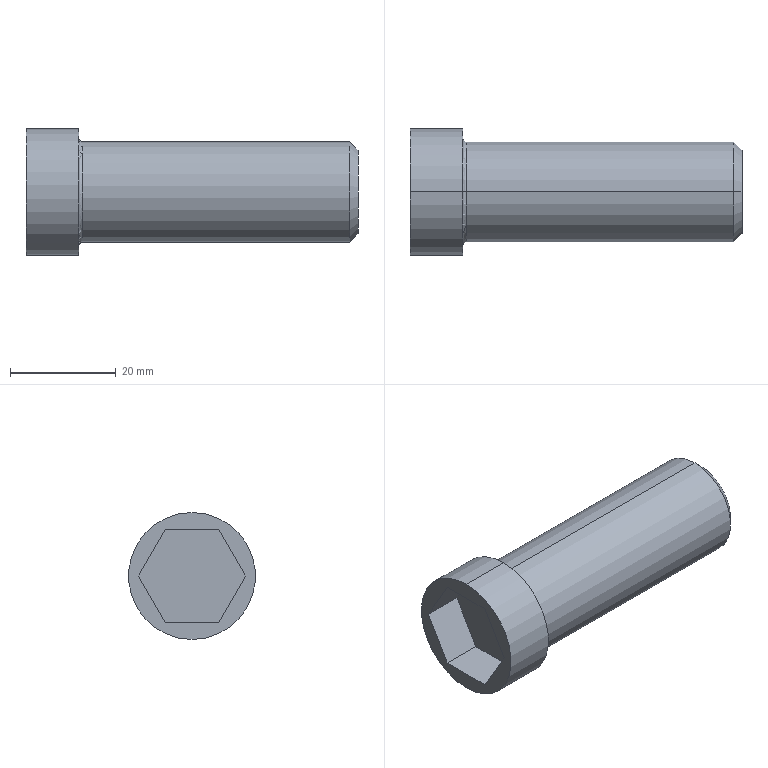Part | SolidWorks | features Chamfer 1, Cut 1, Extrusion 1, Fillet 1, LPattern 1, RevCut 1, Revolution 1 | 1 solid | 18 faces | box 62.8 x 24 x 24 mm | volume 17476 mm3 | plane 10 | cylinder 4 | torus 2 | cone 2 | commonest cylinder face diameters 19.05 x2 24 x2
STEP:
#1=CARTESIAN_POINT('',(10.6,0.,9.525));
#2=VERTEX_POINT('',#1);
#3=CARTESIAN_POINT('',(10.6,0.,-9.525));
#4=VERTEX_POINT('',#3);
#5=CARTESIAN_POINT('',(10.6,0.,0.));
#6=DIRECTION('',(1.,0.,0.));
#7=DIRECTION('',(0.,0.,-1.));
#8=AXIS2_PLACEMENT_3D('',#5,#6,#7);
#9=CIRCLE('',#8,9.525);
#10=EDGE_CURVE('',#2,#4,#9,.T.);
#11=ORIENTED_EDGE('',*,*,#10,.F.);
#12=CARTESIAN_POINT('',(10.,0.,10.125));
#13=VERTEX_POINT('',#12);
#14=CARTESIAN_POINT('',(10.6,0.,10.125));
#15=DIRECTION('',(0.,1.,0.));
#16=DIRECTION('',(0.,0.,1.));
#17=AXIS2_PLACEMENT_3D('',#14,#15,#16);
#18=CIRCLE('',#17,0.6);
#19=EDGE_CURVE('',#2,#13,#18,.T.);
#20=ORIENTED_EDGE('',*,*,#19,.T.);
#21=CARTESIAN_POINT('',(10.,0.,-10.125));
#22=VERTEX_POINT('',#21);
#23=CARTESIAN_POINT('',(10.,0.,0.));
#24=DIRECTION('',(-1.,0.,0.));
#25=DIRECTION('',(0.,0.,-1.));
#26=AXIS2_PLACEMENT_3D('',#23,#24,#25);
#27=CIRCLE('',#26,10.125);
#28=EDGE_CURVE('',#22,#13,#27,.T.);
#29=ORIENTED_EDGE('',*,*,#28,.F.);
#30=CARTESIAN_POINT('',(10.6,0.,-10.125));
#31=DIRECTION('',(0.,-1.,0.));
#32=DIRECTION('',(0.,0.,-1.));
#33=AXIS2_PLACEMENT_3D('',#30,#31,#32);
#34=CIRCLE('',#33,0.6);
#35=EDGE_CURVE('',#4,#22,#34,.T.);
#36=ORIENTED_EDGE('',*,*,#35,.F.);
#37=EDGE_LOOP('',(#11,#20,#29,#36));
#38=FACE_OUTER_BOUND('',#37,.T.);
#39=CARTESIAN_POINT('',(10.6,0.,0.));
#40=DIRECTION('',(1.,0.,0.));
#41=DIRECTION('',(0.,0.,-1.));
#42=AXIS2_PLACEMENT_3D('',#39,#40,#41);
#43=TOROIDAL_SURFACE('',#42,10.125,0.6);
#44=ADVANCED_FACE('',(#38),#43,.F.);
#45=CARTESIAN_POINT('',(62.8,0.,-7.925));
#46=VERTEX_POINT('',#45);
#47=CARTESIAN_POINT('',(62.8,0.,7.925));
#48=VERTEX_POINT('',#47);
#49=CARTESIAN_POINT('',(62.8,0.,0.));
#50=DIRECTION('',(1.,0.,0.));
#51=DIRECTION('',(0.,0.,1.));
#52=AXIS2_PLACEMENT_3D('',#49,#50,#51);
#53=CIRCLE('',#52,7.925);
#54=EDGE_CURVE('',#46,#48,#53,.T.);
#55=ORIENTED_EDGE('',*,*,#54,.F.);
#56=CARTESIAN_POINT('',(61.2,0.,-9.525));
#57=VERTEX_POINT('',#56);
#58=CARTESIAN_POINT('',(61.2,0.,-9.525));
#59=DIRECTION('',(-0.7071,0.,-0.7071));
#60=VECTOR('',#59,1000.);
#61=LINE('',#58,#60);
#62=EDGE_CURVE('',#46,#57,#61,.T.);
#63=ORIENTED_EDGE('',*,*,#62,.T.);
#64=CARTESIAN_POINT('',(61.2,0.,9.525));
#65=VERTEX_POINT('',#64);
#66=CARTESIAN_POINT('',(61.2,0.,0.));
#67=DIRECTION('',(-1.,0.,0.));
#68=DIRECTION('',(0.,0.,1.));
#69=AXIS2_PLACEMENT_3D('',#66,#67,#68);
#70=CIRCLE('',#69,9.525);
#71=EDGE_CURVE('',#65,#57,#70,.T.);
#72=ORIENTED_EDGE('',*,*,#71,.F.);
#73=CARTESIAN_POINT('',(61.2,0.,9.525));
#74=DIRECTION('',(-0.7071,0.,0.7071));
#75=VECTOR('',#74,1000.);
#76=LINE('',#73,#75);
#77=EDGE_CURVE('',#48,#65,#76,.T.);
#78=ORIENTED_EDGE('',*,*,#77,.F.);
#79=EDGE_LOOP('',(#55,#63,#72,#78));
#80=FACE_OUTER_BOUND('',#79,.T.);
#81=CARTESIAN_POINT('',(61.2,0.,0.));
#82=DIRECTION('',(-1.,0.,0.));
#83=DIRECTION('',(0.,0.,1.));
#84=AXIS2_PLACEMENT_3D('',#81,#82,#83);
#85=CONICAL_SURFACE('',#84,9.525,0.7854);
#86=ADVANCED_FACE('',(#80),#85,.T.);
#87=ORIENTED_EDGE('',*,*,#71,.T.);
#88=CARTESIAN_POINT('',(0.,0.,-9.525));
#89=DIRECTION('',(-1.,0.,0.));
#90=VECTOR('',#89,1000.);
#91=LINE('',#88,#90);
#92=EDGE_CURVE('',#57,#4,#91,.T.);
#93=ORIENTED_EDGE('',*,*,#92,.T.);
#94=CARTESIAN_POINT('',(10.6,0.,0.));
#95=DIRECTION('',(1.,0.,0.));
#96=DIRECTION('',(0.,0.,-1.));
#97=AXIS2_PLACEMENT_3D('',#94,#95,#96);
#98=CIRCLE('',#97,9.525);
#99=EDGE_CURVE('',#4,#2,#98,.T.);
#100=ORIENTED_EDGE('',*,*,#99,.T.);
#101=CARTESIAN_POINT('',(0.,0.,9.525));
#102=DIRECTION('',(-1.,0.,0.));
#103=VECTOR('',#102,1000.);
#104=LINE('',#101,#103);
#105=EDGE_CURVE('',#65,#2,#104,.T.);
#106=ORIENTED_EDGE('',*,*,#105,.F.);
#107=EDGE_LOOP('',(#87,#93,#100,#106));
#108=FACE_OUTER_BOUND('',#107,.T.);
#109=CARTESIAN_POINT('',(0.,0.,0.));
#110=DIRECTION('',(-1.,0.,0.));
#111=DIRECTION('',(0.,0.,1.));
#112=AXIS2_PLACEMENT_3D('',#109,#110,#111);
#113=CYLINDRICAL_SURFACE('',#112,9.525);
#114=ADVANCED_FACE('',(#108),#113,.T.);
#115=CARTESIAN_POINT('',(10.,0.,-12.));
#116=VERTEX_POINT('',#115);
#117=CARTESIAN_POINT('',(10.,0.,12.));
#118=VERTEX_POINT('',#117);
#119=CARTESIAN_POINT('',(10.,0.,0.));
#120=DIRECTION('',(1.,0.,0.));
#121=DIRECTION('',(0.,0.,-1.));
#122=AXIS2_PLACEMENT_3D('',#119,#120,#121);
#123=CIRCLE('',#122,12.);
#124=EDGE_CURVE('',#116,#118,#123,.T.);
#125=ORIENTED_EDGE('',*,*,#124,.F.);
#126=CARTESIAN_POINT('',(0.,0.,-12.));
#127=VERTEX_POINT('',#126);
#128=CARTESIAN_POINT('',(10.,0.,-12.));
#129=DIRECTION('',(-1.,0.,0.));
#130=VECTOR('',#129,1000.);
#131=LINE('',#128,#130);
#132=EDGE_CURVE('',#116,#127,#131,.T.);
#133=ORIENTED_EDGE('',*,*,#132,.T.);
#134=CARTESIAN_POINT('',(0.,0.,12.));
#135=VERTEX_POINT('',#134);
#136=CARTESIAN_POINT('',(0.,0.,0.));
#137=DIRECTION('',(1.,0.,0.));
#138=DIRECTION('',(0.,0.,-1.));
#139=AXIS2_PLACEMENT_3D('',#136,#137,#138);
#140=CIRCLE('',#139,12.);
#141=EDGE_CURVE('',#127,#135,#140,.T.);
#142=ORIENTED_EDGE('',*,*,#141,.T.);
#143=CARTESIAN_POINT('',(10.,0.,12.));
#144=DIRECTION('',(-1.,0.,0.));
#145=VECTOR('',#144,1000.);
#146=LINE('',#143,#145);
#147=EDGE_CURVE('',#118,#135,#146,.T.);
#148=ORIENTED_EDGE('',*,*,#147,.F.);
#149=EDGE_LOOP('',(#125,#133,#142,#148));
#150=FACE_OUTER_BOUND('',#149,.T.);
#151=CARTESIAN_POINT('',(10.,0.,0.));
#152=DIRECTION('',(-1.,0.,0.));
#153=DIRECTION('',(0.,0.,1.));
#154=AXIS2_PLACEMENT_3D('',#151,#152,#153);
#155=CYLINDRICAL_SURFACE('',#154,12.);
#156=ADVANCED_FACE('',(#150),#155,.T.);
#157=ORIENTED_EDGE('',*,*,#28,.T.);
#158=CARTESIAN_POINT('',(10.,0.,0.));
#159=DIRECTION('',(-1.,0.,0.));
#160=DIRECTION('',(0.,0.,-1.));
#161=AXIS2_PLACEMENT_3D('',#158,#159,#160);
#162=CIRCLE('',#161,10.125);
#163=EDGE_CURVE('',#13,#22,#162,.T.);
#164=ORIENTED_EDGE('',*,*,#163,.T.);
#165=EDGE_LOOP('',(#157,#164));
#166=FACE_BOUND('',#165,.T.);
#167=CARTESIAN_POINT('',(10.,0.,0.));
#168=DIRECTION('',(1.,0.,0.));
#169=DIRECTION('',(0.,0.,-1.));
#170=AXIS2_PLACEMENT_3D('',#167,#168,#169);
#171=CIRCLE('',#170,12.);
#172=EDGE_CURVE('',#118,#116,#171,.T.);
#173=ORIENTED_EDGE('',*,*,#172,.T.);
#174=ORIENTED_EDGE('',*,*,#124,.T.);
#175=EDGE_LOOP('',(#173,#174));
#176=FACE_OUTER_BOUND('',#175,.T.);
#177=CARTESIAN_POINT('',(10.,0.,0.));
#178=DIRECTION('',(1.,0.,0.));
#179=DIRECTION('',(0.,0.,-1.));
#180=AXIS2_PLACEMENT_3D('',#177,#178,#179);
#181=PLANE('',#180);
#182=ADVANCED_FACE('',(#166,#176),#181,.T.);
#183=ORIENTED_EDGE('',*,*,#132,.F.);
#184=ORIENTED_EDGE('',*,*,#172,.F.);
#185=ORIENTED_EDGE('',*,*,#147,.T.);
#186=CARTESIAN_POINT('',(0.,0.,0.));
#187=DIRECTION('',(1.,0.,0.));
#188=DIRECTION('',(0.,0.,-1.));
#189=AXIS2_PLACEMENT_3D('',#186,#187,#188);
#190=CIRCLE('',#189,12.);
#191=EDGE_CURVE('',#135,#127,#190,.T.);
#192=ORIENTED_EDGE('',*,*,#191,.T.);
#193=EDGE_LOOP('',(#183,#184,#185,#192));
#194=FACE_OUTER_BOUND('',#193,.T.);
#195=CARTESIAN_POINT('',(10.,0.,0.));
#196=DIRECTION('',(-1.,0.,0.));
#197=DIRECTION('',(0.,0.,1.));
#198=AXIS2_PLACEMENT_3D('',#195,#196,#197);
#199=CYLINDRICAL_SURFACE('',#198,12.);
#200=ADVANCED_FACE('',(#194),#199,.T.);
#201=CARTESIAN_POINT('',(0.,5.062,-8.768));
#202=VERTEX_POINT('',#201);
#203=CARTESIAN_POINT('',(0.,-5.062,-8.768));
#204=VERTEX_POINT('',#203);
#205=CARTESIAN_POINT('',(0.,5.062,-8.768));
#206=DIRECTION('',(0.,-1.,0.));
#207=VECTOR('',#206,1000.);
#208=LINE('',#205,#207);
#209=EDGE_CURVE('',#202,#204,#208,.T.);
#210=ORIENTED_EDGE('',*,*,#209,.F.);
#211=CARTESIAN_POINT('',(0.,10.124,0.));
#212=VERTEX_POINT('',#211);
#213=CARTESIAN_POINT('',(0.,10.124,0.));
#214=DIRECTION('',(0.,-0.5,-0.866));
#215=VECTOR('',#214,1000.);
#216=LINE('',#213,#215);
#217=EDGE_CURVE('',#212,#202,#216,.T.);
#218=ORIENTED_EDGE('',*,*,#217,.F.);
#219=CARTESIAN_POINT('',(0.,5.062,8.768));
#220=VERTEX_POINT('',#219);
#221=CARTESIAN_POINT('',(0.,5.062,8.768));
#222=DIRECTION('',(0.,0.5,-0.866));
#223=VECTOR('',#222,1000.);
#224=LINE('',#221,#223);
#225=EDGE_CURVE('',#220,#212,#224,.T.);
#226=ORIENTED_EDGE('',*,*,#225,.F.);
#227=CARTESIAN_POINT('',(0.,-5.062,8.768));
#228=VERTEX_POINT('',#227);
#229=CARTESIAN_POINT('',(0.,-5.062,8.768));
#230=DIRECTION('',(0.,1.,0.));
#231=VECTOR('',#230,1000.);
#232=LINE('',#229,#231);
#233=EDGE_CURVE('',#228,#220,#232,.T.);
#234=ORIENTED_EDGE('',*,*,#233,.F.);
#235=CARTESIAN_POINT('',(0.,-10.124,0.));
#236=VERTEX_POINT('',#235);
#237=CARTESIAN_POINT('',(0.,-10.124,0.));
#238=DIRECTION('',(0.,0.5,0.866));
#239=VECTOR('',#238,1000.);
#240=LINE('',#237,#239);
#241=EDGE_CURVE('',#236,#228,#240,.T.);
#242=ORIENTED_EDGE('',*,*,#241,.F.);
#243=CARTESIAN_POINT('',(0.,-5.062,-8.768));
#244=DIRECTION('',(0.,-0.5,0.866));
#245=VECTOR('',#244,1000.);
#246=LINE('',#243,#245);
#247=EDGE_CURVE('',#204,#236,#246,.T.);
#248=ORIENTED_EDGE('',*,*,#247,.F.);
#249=EDGE_LOOP('',(#210,#218,#226,#234,#242,#248));
#250=FACE_BOUND('',#249,.T.);
#251=ORIENTED_EDGE('',*,*,#191,.F.);
#252=ORIENTED_EDGE('',*,*,#141,.F.);
#253=EDGE_LOOP('',(#251,#252));
#254=FACE_OUTER_BOUND('',#253,.T.);
#255=CARTESIAN_POINT('',(0.,0.,0.));
#256=DIRECTION('',(1.,0.,0.));
#257=DIRECTION('',(0.,0.,-1.));
#258=AXIS2_PLACEMENT_3D('',#255,#256,#257);
#259=PLANE('',#258);
#260=ADVANCED_FACE('',(#250,#254),#259,.F.);
#261=ORIENTED_EDGE('',*,*,#92,.F.);
#262=CARTESIAN_POINT('',(61.2,0.,0.));
#263=DIRECTION('',(-1.,0.,0.));
#264=DIRECTION('',(0.,0.,1.));
#265=AXIS2_PLACEMENT_3D('',#262,#263,#264);
#266=CIRCLE('',#265,9.525);
#267=EDGE_CURVE('',#57,#65,#266,.T.);
#268=ORIENTED_EDGE('',*,*,#267,.T.);
#269=ORIENTED_EDGE('',*,*,#105,.T.);
#270=ORIENTED_EDGE('',*,*,#10,.T.);
#271=EDGE_LOOP('',(#261,#268,#269,#270));
#272=FACE_OUTER_BOUND('',#271,.T.);
#273=CARTESIAN_POINT('',(0.,0.,0.));
#274=DIRECTION('',(-1.,0.,0.));
#275=DIRECTION('',(0.,0.,1.));
#276=AXIS2_PLACEMENT_3D('',#273,#274,#275);
#277=CYLINDRICAL_SURFACE('',#276,9.525);
#278=ADVANCED_FACE('',(#272),#277,.T.);
#279=CARTESIAN_POINT('',(62.8,0.,0.));
#280=DIRECTION('',(1.,0.,0.));
#281=DIRECTION('',(0.,0.,1.));
#282=AXIS2_PLACEMENT_3D('',#279,#280,#281);
#283=CIRCLE('',#282,7.925);
#284=EDGE_CURVE('',#48,#46,#283,.T.);
#285=ORIENTED_EDGE('',*,*,#284,.T.);
#286=ORIENTED_EDGE('',*,*,#54,.T.);
#287=EDGE_LOOP('',(#285,#286));
#288=FACE_OUTER_BOUND('',#287,.T.);
#289=CARTESIAN_POINT('',(62.8,0.,0.));
#290=DIRECTION('',(-1.,0.,0.));
#291=DIRECTION('',(0.,0.,1.));
#292=AXIS2_PLACEMENT_3D('',#289,#290,#291);
#293=PLANE('',#292);
#294=ADVANCED_FACE('',(#288),#293,.F.);
#295=ORIENTED_EDGE('',*,*,#62,.F.);
#296=ORIENTED_EDGE('',*,*,#284,.F.);
#297=ORIENTED_EDGE('',*,*,#77,.T.);
#298=ORIENTED_EDGE('',*,*,#267,.F.);
#299=EDGE_LOOP('',(#295,#296,#297,#298));
#300=FACE_OUTER_BOUND('',#299,.T.);
#301=CARTESIAN_POINT('',(61.2,0.,0.));
#302=DIRECTION('',(-1.,0.,0.));
#303=DIRECTION('',(0.,0.,1.));
#304=AXIS2_PLACEMENT_3D('',#301,#302,#303);
#305=CONICAL_SURFACE('',#304,9.525,0.7854);
#306=ADVANCED_FACE('',(#300),#305,.T.);
#307=ORIENTED_EDGE('',*,*,#19,.F.);
#308=ORIENTED_EDGE('',*,*,#99,.F.);
#309=ORIENTED_EDGE('',*,*,#35,.T.);
#310=ORIENTED_EDGE('',*,*,#163,.F.);
#311=EDGE_LOOP('',(#307,#308,#309,#310));
#312=FACE_OUTER_BOUND('',#311,.T.);
#313=CARTESIAN_POINT('',(10.6,0.,0.));
#314=DIRECTION('',(1.,0.,0.));
#315=DIRECTION('',(0.,0.,-1.));
#316=AXIS2_PLACEMENT_3D('',#313,#314,#315);
#317=TOROIDAL_SURFACE('',#316,10.125,0.6);
#318=ADVANCED_FACE('',(#312),#317,.F.);
#319=ORIENTED_EDGE('',*,*,#217,.T.);
#320=CARTESIAN_POINT('',(7.62,5.062,-8.768));
#321=VERTEX_POINT('',#320);
#322=CARTESIAN_POINT('',(7.62,5.062,-8.768));
#323=DIRECTION('',(-1.,0.,0.));
#324=VECTOR('',#323,1000.);
#325=LINE('',#322,#324);
#326=EDGE_CURVE('',#321,#202,#325,.T.);
#327=ORIENTED_EDGE('',*,*,#326,.F.);
#328=CARTESIAN_POINT('',(7.62,10.124,0.));
#329=VERTEX_POINT('',#328);
#330=CARTESIAN_POINT('',(7.62,10.124,0.));
#331=DIRECTION('',(0.,-0.5,-0.866));
#332=VECTOR('',#331,1000.);
#333=LINE('',#330,#332);
#334=EDGE_CURVE('',#329,#321,#333,.T.);
#335=ORIENTED_EDGE('',*,*,#334,.F.);
#336=CARTESIAN_POINT('',(7.62,10.124,0.));
#337=DIRECTION('',(-1.,0.,0.));
#338=VECTOR('',#337,1000.);
#339=LINE('',#336,#338);
#340=EDGE_CURVE('',#329,#212,#339,.T.);
#341=ORIENTED_EDGE('',*,*,#340,.T.);
#342=EDGE_LOOP('',(#319,#327,#335,#341));
#343=FACE_OUTER_BOUND('',#342,.T.);
#344=CARTESIAN_POINT('',(7.62,10.124,0.));
#345=DIRECTION('',(0.,0.866,-0.5));
#346=DIRECTION('',(0.,0.5,0.866));
#347=AXIS2_PLACEMENT_3D('',#344,#345,#346);
#348=PLANE('',#347);
#349=ADVANCED_FACE('',(#343),#348,.F.);
#350=ORIENTED_EDGE('',*,*,#225,.T.);
#351=ORIENTED_EDGE('',*,*,#340,.F.);
#352=CARTESIAN_POINT('',(7.62,5.062,8.768));
#353=VERTEX_POINT('',#352);
#354=CARTESIAN_POINT('',(7.62,5.062,8.768));
#355=DIRECTION('',(0.,0.5,-0.866));
#356=VECTOR('',#355,1000.);
#357=LINE('',#354,#356);
#358=EDGE_CURVE('',#353,#329,#357,.T.);
#359=ORIENTED_EDGE('',*,*,#358,.F.);
#360=CARTESIAN_POINT('',(7.62,5.062,8.768));
#361=DIRECTION('',(-1.,0.,0.));
#362=VECTOR('',#361,1000.);
#363=LINE('',#360,#362);
#364=EDGE_CURVE('',#353,#220,#363,.T.);
#365=ORIENTED_EDGE('',*,*,#364,.T.);
#366=EDGE_LOOP('',(#350,#351,#359,#365));
#367=FACE_OUTER_BOUND('',#366,.T.);
#368=CARTESIAN_POINT('',(7.62,5.062,8.768));
#369=DIRECTION('',(0.,0.866,0.5));
#370=DIRECTION('',(0.,-0.5,0.866));
#371=AXIS2_PLACEMENT_3D('',#368,#369,#370);
#372=PLANE('',#371);
#373=ADVANCED_FACE('',(#367),#372,.F.);
#374=ORIENTED_EDGE('',*,*,#233,.T.);
#375=ORIENTED_EDGE('',*,*,#364,.F.);
#376=CARTESIAN_POINT('',(7.62,-5.062,8.768));
#377=VERTEX_POINT('',#376);
#378=CARTESIAN_POINT('',(7.62,-5.062,8.768));
#379=DIRECTION('',(0.,1.,0.));
#380=VECTOR('',#379,1000.);
#381=LINE('',#378,#380);
#382=EDGE_CURVE('',#377,#353,#381,.T.);
#383=ORIENTED_EDGE('',*,*,#382,.F.);
#384=CARTESIAN_POINT('',(7.62,-5.062,8.768));
#385=DIRECTION('',(-1.,0.,0.));
#386=VECTOR('',#385,1000.);
#387=LINE('',#384,#386);
#388=EDGE_CURVE('',#377,#228,#387,.T.);
#389=ORIENTED_EDGE('',*,*,#388,.T.);
#390=EDGE_LOOP('',(#374,#375,#383,#389));
#391=FACE_OUTER_BOUND('',#390,.T.);
#392=CARTESIAN_POINT('',(7.62,-5.062,8.768));
#393=DIRECTION('',(0.,0.,1.));
#394=DIRECTION('',(1.,0.,0.));
#395=AXIS2_PLACEMENT_3D('',#392,#393,#394);
#396=PLANE('',#395);
#397=ADVANCED_FACE('',(#391),#396,.F.);
#398=ORIENTED_EDGE('',*,*,#241,.T.);
#399=ORIENTED_EDGE('',*,*,#388,.F.);
#400=CARTESIAN_POINT('',(7.62,-10.124,0.));
#401=VERTEX_POINT('',#400);
#402=CARTESIAN_POINT('',(7.62,-10.124,0.));
#403=DIRECTION('',(0.,0.5,0.866));
#404=VECTOR('',#403,1000.);
#405=LINE('',#402,#404);
#406=EDGE_CURVE('',#401,#377,#405,.T.);
#407=ORIENTED_EDGE('',*,*,#406,.F.);
#408=CARTESIAN_POINT('',(7.62,-10.124,0.));
#409=DIRECTION('',(-1.,0.,0.));
#410=VECTOR('',#409,1000.);
#411=LINE('',#408,#410);
#412=EDGE_CURVE('',#401,#236,#411,.T.);
#413=ORIENTED_EDGE('',*,*,#412,.T.);
#414=EDGE_LOOP('',(#398,#399,#407,#413));
#415=FACE_OUTER_BOUND('',#414,.T.);
#416=CARTESIAN_POINT('',(7.62,-10.124,0.));
#417=DIRECTION('',(0.,-0.866,0.5));
#418=DIRECTION('',(0.,-0.5,-0.866));
#419=AXIS2_PLACEMENT_3D('',#416,#417,#418);
#420=PLANE('',#419);
#421=ADVANCED_FACE('',(#415),#420,.F.);
#422=ORIENTED_EDGE('',*,*,#247,.T.);
#423=ORIENTED_EDGE('',*,*,#412,.F.);
#424=CARTESIAN_POINT('',(7.62,-5.062,-8.768));
#425=VERTEX_POINT('',#424);
#426=CARTESIAN_POINT('',(7.62,-5.062,-8.768));
#427=DIRECTION('',(0.,-0.5,0.866));
#428=VECTOR('',#427,1000.);
#429=LINE('',#426,#428);
#430=EDGE_CURVE('',#425,#401,#429,.T.);
#431=ORIENTED_EDGE('',*,*,#430,.F.);
#432=CARTESIAN_POINT('',(7.62,-5.062,-8.768));
#433=DIRECTION('',(-1.,0.,0.));
#434=VECTOR('',#433,1000.);
#435=LINE('',#432,#434);
#436=EDGE_CURVE('',#425,#204,#435,.T.);
#437=ORIENTED_EDGE('',*,*,#436,.T.);
#438=EDGE_LOOP('',(#422,#423,#431,#437));
#439=FACE_OUTER_BOUND('',#438,.T.);
#440=CARTESIAN_POINT('',(7.62,-5.062,-8.768));
#441=DIRECTION('',(0.,-0.866,-0.5));
#442=DIRECTION('',(0.,0.5,-0.866));
#443=AXIS2_PLACEMENT_3D('',#440,#441,#442);
#444=PLANE('',#443);
#445=ADVANCED_FACE('',(#439),#444,.F.);
#446=ORIENTED_EDGE('',*,*,#209,.T.);
#447=ORIENTED_EDGE('',*,*,#436,.F.);
#448=CARTESIAN_POINT('',(7.62,5.062,-8.768));
#449=DIRECTION('',(0.,-1.,0.));
#450=VECTOR('',#449,1000.);
#451=LINE('',#448,#450);
#452=EDGE_CURVE('',#321,#425,#451,.T.);
#453=ORIENTED_EDGE('',*,*,#452,.F.);
#454=ORIENTED_EDGE('',*,*,#326,.T.);
#455=EDGE_LOOP('',(#446,#447,#453,#454));
#456=FACE_OUTER_BOUND('',#455,.T.);
#457=CARTESIAN_POINT('',(7.62,5.062,-8.768));
#458=DIRECTION('',(0.,0.,-1.));
#459=DIRECTION('',(0.,1.,0.));
#460=AXIS2_PLACEMENT_3D('',#457,#458,#459);
#461=PLANE('',#460);
#462=ADVANCED_FACE('',(#456),#461,.F.);
#463=ORIENTED_EDGE('',*,*,#334,.T.);
#464=ORIENTED_EDGE('',*,*,#452,.T.);
#465=ORIENTED_EDGE('',*,*,#430,.T.);
#466=ORIENTED_EDGE('',*,*,#406,.T.);
#467=ORIENTED_EDGE('',*,*,#382,.T.);
#468=ORIENTED_EDGE('',*,*,#358,.T.);
#469=EDGE_LOOP('',(#463,#464,#465,#466,#467,#468));
#470=FACE_OUTER_BOUND('',#469,.T.);
#471=CARTESIAN_POINT('',(7.62,0.,-17.536));
#472=DIRECTION('',(-1.,0.,0.));
#473=DIRECTION('',(0.,0.,1.));
#474=AXIS2_PLACEMENT_3D('',#471,#472,#473);
#475=PLANE('',#474);
#476=ADVANCED_FACE('',(#470),#475,.T.);
#477=CLOSED_SHELL('',(#44,#86,#114,#156,#182,#200,#260,#278,#294,#306,#318,#349,#373,#397,#421,#445,#462,#476));
#478=MANIFOLD_SOLID_BREP('',#477);
#479=CARTESIAN_POINT('',(0.,0.,0.));
#480=DIRECTION('',(0.,0.,1.));
#481=DIRECTION('',(1.,0.,0.));
#482=AXIS2_PLACEMENT_3D('',#479,#480,#481);
#483=(LENGTH_UNIT()NAMED_UNIT(*)SI_UNIT(.MILLI.,.METRE.));
#484=UNCERTAINTY_MEASURE_WITH_UNIT(LENGTH_MEASURE(0.00001),#483,'','');
#485=(NAMED_UNIT(*)PLANE_ANGLE_UNIT()SI_UNIT($,.RADIAN.));
#486=(NAMED_UNIT(*)SI_UNIT($,.STERADIAN.)SOLID_ANGLE_UNIT());
#487=(GEOMETRIC_REPRESENTATION_CONTEXT(3)GLOBAL_UNCERTAINTY_ASSIGNED_CONTEXT((#484))GLOBAL_UNIT_ASSIGNED_CONTEXT((#483,#485,#486))REPRESENTATION_CONTEXT('',''));
#488=ADVANCED_BREP_SHAPE_REPRESENTATION('',(#478,#482),#487);